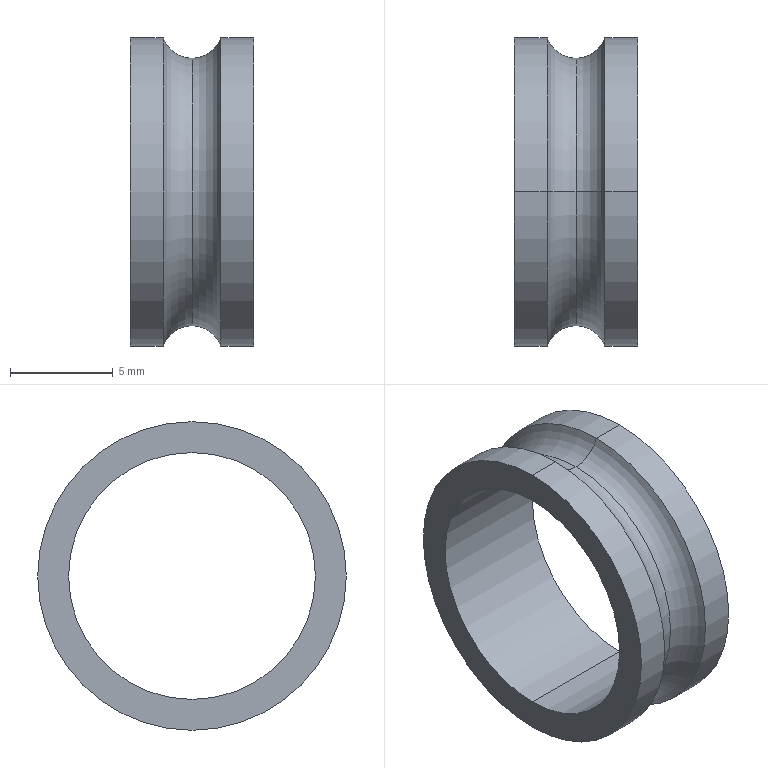Part | SolidWorks | features Revolution 1 | 1 solid | 12 faces | box 6 x 15 x 15 mm | volume 290.652 mm3 | cylinder 6 | torus 4 | plane 2 | commonest cylinder face diameters 15 x4 12 x2
STEP:
#1=CARTESIAN_POINT('',(1.6,0.,7.5));
#2=VERTEX_POINT('',#1);
#3=CARTESIAN_POINT('',(3.,0.,6.5));
#4=VERTEX_POINT('',#3);
#5=CARTESIAN_POINT('',(3.,0.,7.98));
#6=DIRECTION('',(0.,-1.,0.));
#7=DIRECTION('',(0.,0.,-1.));
#8=AXIS2_PLACEMENT_3D('',#5,#6,#7);
#9=CIRCLE('',#8,1.48);
#10=EDGE_CURVE('',#2,#4,#9,.T.);
#11=ORIENTED_EDGE('',*,*,#10,.T.);
#12=CARTESIAN_POINT('',(3.,0.,-6.5));
#13=VERTEX_POINT('',#12);
#14=CARTESIAN_POINT('',(3.,0.,0.));
#15=DIRECTION('',(-1.,0.,0.));
#16=DIRECTION('',(0.,0.,1.));
#17=AXIS2_PLACEMENT_3D('',#14,#15,#16);
#18=CIRCLE('',#17,6.5);
#19=EDGE_CURVE('',#4,#13,#18,.T.);
#20=ORIENTED_EDGE('',*,*,#19,.T.);
#21=CARTESIAN_POINT('',(1.6,0.,-7.5));
#22=VERTEX_POINT('',#21);
#23=CARTESIAN_POINT('',(3.,0.,-7.98));
#24=DIRECTION('',(0.,1.,0.));
#25=DIRECTION('',(0.,0.,1.));
#26=AXIS2_PLACEMENT_3D('',#23,#24,#25);
#27=CIRCLE('',#26,1.48);
#28=EDGE_CURVE('',#22,#13,#27,.T.);
#29=ORIENTED_EDGE('',*,*,#28,.F.);
#30=CARTESIAN_POINT('',(1.6,0.,0.));
#31=DIRECTION('',(-1.,0.,0.));
#32=DIRECTION('',(0.,0.,1.));
#33=AXIS2_PLACEMENT_3D('',#30,#31,#32);
#34=CIRCLE('',#33,7.5);
#35=EDGE_CURVE('',#2,#22,#34,.T.);
#36=ORIENTED_EDGE('',*,*,#35,.F.);
#37=EDGE_LOOP('',(#11,#20,#29,#36));
#38=FACE_OUTER_BOUND('',#37,.T.);
#39=CARTESIAN_POINT('',(3.,0.,0.));
#40=DIRECTION('',(-1.,0.,0.));
#41=DIRECTION('',(0.,0.,1.));
#42=AXIS2_PLACEMENT_3D('',#39,#40,#41);
#43=TOROIDAL_SURFACE('',#42,7.98,1.48);
#44=ADVANCED_FACE('',(#38),#43,.F.);
#45=ORIENTED_EDGE('',*,*,#28,.T.);
#46=CARTESIAN_POINT('',(3.,0.,0.));
#47=DIRECTION('',(-1.,0.,0.));
#48=DIRECTION('',(0.,0.,1.));
#49=AXIS2_PLACEMENT_3D('',#46,#47,#48);
#50=CIRCLE('',#49,6.5);
#51=EDGE_CURVE('',#13,#4,#50,.T.);
#52=ORIENTED_EDGE('',*,*,#51,.T.);
#53=ORIENTED_EDGE('',*,*,#10,.F.);
#54=CARTESIAN_POINT('',(1.6,0.,0.));
#55=DIRECTION('',(-1.,0.,0.));
#56=DIRECTION('',(0.,0.,1.));
#57=AXIS2_PLACEMENT_3D('',#54,#55,#56);
#58=CIRCLE('',#57,7.5);
#59=EDGE_CURVE('',#22,#2,#58,.T.);
#60=ORIENTED_EDGE('',*,*,#59,.F.);
#61=EDGE_LOOP('',(#45,#52,#53,#60));
#62=FACE_OUTER_BOUND('',#61,.T.);
#63=CARTESIAN_POINT('',(3.,0.,0.));
#64=DIRECTION('',(-1.,0.,0.));
#65=DIRECTION('',(0.,0.,1.));
#66=AXIS2_PLACEMENT_3D('',#63,#64,#65);
#67=TOROIDAL_SURFACE('',#66,7.98,1.48);
#68=ADVANCED_FACE('',(#62),#67,.F.);
#69=ORIENTED_EDGE('',*,*,#35,.T.);
#70=CARTESIAN_POINT('',(0.,0.,-7.5));
#71=VERTEX_POINT('',#70);
#72=CARTESIAN_POINT('',(0.,0.,-7.5));
#73=DIRECTION('',(-1.,0.,0.));
#74=VECTOR('',#73,1000.);
#75=LINE('',#72,#74);
#76=EDGE_CURVE('',#22,#71,#75,.T.);
#77=ORIENTED_EDGE('',*,*,#76,.T.);
#78=CARTESIAN_POINT('',(0.,0.,7.5));
#79=VERTEX_POINT('',#78);
#80=CARTESIAN_POINT('',(0.,0.,0.));
#81=DIRECTION('',(-1.,0.,0.));
#82=DIRECTION('',(0.,0.,1.));
#83=AXIS2_PLACEMENT_3D('',#80,#81,#82);
#84=CIRCLE('',#83,7.5);
#85=EDGE_CURVE('',#79,#71,#84,.T.);
#86=ORIENTED_EDGE('',*,*,#85,.F.);
#87=CARTESIAN_POINT('',(0.,0.,7.5));
#88=DIRECTION('',(-1.,0.,0.));
#89=VECTOR('',#88,1000.);
#90=LINE('',#87,#89);
#91=EDGE_CURVE('',#2,#79,#90,.T.);
#92=ORIENTED_EDGE('',*,*,#91,.F.);
#93=EDGE_LOOP('',(#69,#77,#86,#92));
#94=FACE_OUTER_BOUND('',#93,.T.);
#95=CARTESIAN_POINT('',(0.,0.,0.));
#96=DIRECTION('',(-1.,0.,0.));
#97=DIRECTION('',(0.,0.,1.));
#98=AXIS2_PLACEMENT_3D('',#95,#96,#97);
#99=CYLINDRICAL_SURFACE('',#98,7.5);
#100=ADVANCED_FACE('',(#94),#99,.T.);
#101=ORIENTED_EDGE('',*,*,#51,.F.);
#102=CARTESIAN_POINT('',(4.4,0.,-7.5));
#103=VERTEX_POINT('',#102);
#104=CARTESIAN_POINT('',(3.,0.,-7.98));
#105=DIRECTION('',(0.,1.,0.));
#106=DIRECTION('',(0.,0.,1.));
#107=AXIS2_PLACEMENT_3D('',#104,#105,#106);
#108=CIRCLE('',#107,1.48);
#109=EDGE_CURVE('',#13,#103,#108,.T.);
#110=ORIENTED_EDGE('',*,*,#109,.T.);
#111=CARTESIAN_POINT('',(4.4,0.,7.5));
#112=VERTEX_POINT('',#111);
#113=CARTESIAN_POINT('',(4.4,0.,0.));
#114=DIRECTION('',(-1.,0.,0.));
#115=DIRECTION('',(0.,0.,1.));
#116=AXIS2_PLACEMENT_3D('',#113,#114,#115);
#117=CIRCLE('',#116,7.5);
#118=EDGE_CURVE('',#103,#112,#117,.T.);
#119=ORIENTED_EDGE('',*,*,#118,.T.);
#120=CARTESIAN_POINT('',(3.,0.,7.98));
#121=DIRECTION('',(0.,-1.,0.));
#122=DIRECTION('',(0.,0.,-1.));
#123=AXIS2_PLACEMENT_3D('',#120,#121,#122);
#124=CIRCLE('',#123,1.48);
#125=EDGE_CURVE('',#4,#112,#124,.T.);
#126=ORIENTED_EDGE('',*,*,#125,.F.);
#127=EDGE_LOOP('',(#101,#110,#119,#126));
#128=FACE_OUTER_BOUND('',#127,.T.);
#129=CARTESIAN_POINT('',(3.,0.,0.));
#130=DIRECTION('',(-1.,0.,0.));
#131=DIRECTION('',(0.,0.,1.));
#132=AXIS2_PLACEMENT_3D('',#129,#130,#131);
#133=TOROIDAL_SURFACE('',#132,7.98,1.48);
#134=ADVANCED_FACE('',(#128),#133,.F.);
#135=CARTESIAN_POINT('',(6.,0.,7.5));
#136=VERTEX_POINT('',#135);
#137=CARTESIAN_POINT('',(6.,0.,-7.5));
#138=VERTEX_POINT('',#137);
#139=CARTESIAN_POINT('',(6.,0.,0.));
#140=DIRECTION('',(-1.,0.,0.));
#141=DIRECTION('',(0.,0.,1.));
#142=AXIS2_PLACEMENT_3D('',#139,#140,#141);
#143=CIRCLE('',#142,7.5);
#144=EDGE_CURVE('',#136,#138,#143,.T.);
#145=ORIENTED_EDGE('',*,*,#144,.T.);
#146=CARTESIAN_POINT('',(0.,0.,-7.5));
#147=DIRECTION('',(-1.,0.,0.));
#148=VECTOR('',#147,1000.);
#149=LINE('',#146,#148);
#150=EDGE_CURVE('',#138,#103,#149,.T.);
#151=ORIENTED_EDGE('',*,*,#150,.T.);
#152=CARTESIAN_POINT('',(4.4,0.,0.));
#153=DIRECTION('',(-1.,0.,0.));
#154=DIRECTION('',(0.,0.,1.));
#155=AXIS2_PLACEMENT_3D('',#152,#153,#154);
#156=CIRCLE('',#155,7.5);
#157=EDGE_CURVE('',#112,#103,#156,.T.);
#158=ORIENTED_EDGE('',*,*,#157,.F.);
#159=CARTESIAN_POINT('',(0.,0.,7.5));
#160=DIRECTION('',(-1.,0.,0.));
#161=VECTOR('',#160,1000.);
#162=LINE('',#159,#161);
#163=EDGE_CURVE('',#136,#112,#162,.T.);
#164=ORIENTED_EDGE('',*,*,#163,.F.);
#165=EDGE_LOOP('',(#145,#151,#158,#164));
#166=FACE_OUTER_BOUND('',#165,.T.);
#167=CARTESIAN_POINT('',(0.,0.,0.));
#168=DIRECTION('',(-1.,0.,0.));
#169=DIRECTION('',(0.,0.,1.));
#170=AXIS2_PLACEMENT_3D('',#167,#168,#169);
#171=CYLINDRICAL_SURFACE('',#170,7.5);
#172=ADVANCED_FACE('',(#166),#171,.T.);
#173=CARTESIAN_POINT('',(6.,0.,-6.));
#174=VERTEX_POINT('',#173);
#175=CARTESIAN_POINT('',(6.,0.,6.));
#176=VERTEX_POINT('',#175);
#177=CARTESIAN_POINT('',(6.,0.,0.));
#178=DIRECTION('',(-1.,0.,0.));
#179=DIRECTION('',(0.,0.,1.));
#180=AXIS2_PLACEMENT_3D('',#177,#178,#179);
#181=CIRCLE('',#180,6.);
#182=EDGE_CURVE('',#174,#176,#181,.T.);
#183=ORIENTED_EDGE('',*,*,#182,.F.);
#184=CARTESIAN_POINT('',(0.,0.,-6.));
#185=VERTEX_POINT('',#184);
#186=CARTESIAN_POINT('',(0.,0.,-6.));
#187=DIRECTION('',(-1.,0.,0.));
#188=VECTOR('',#187,1000.);
#189=LINE('',#186,#188);
#190=EDGE_CURVE('',#174,#185,#189,.T.);
#191=ORIENTED_EDGE('',*,*,#190,.T.);
#192=CARTESIAN_POINT('',(0.,0.,6.));
#193=VERTEX_POINT('',#192);
#194=CARTESIAN_POINT('',(0.,0.,0.));
#195=DIRECTION('',(-1.,0.,0.));
#196=DIRECTION('',(0.,0.,1.));
#197=AXIS2_PLACEMENT_3D('',#194,#195,#196);
#198=CIRCLE('',#197,6.);
#199=EDGE_CURVE('',#185,#193,#198,.T.);
#200=ORIENTED_EDGE('',*,*,#199,.T.);
#201=CARTESIAN_POINT('',(0.,0.,6.));
#202=DIRECTION('',(-1.,0.,0.));
#203=VECTOR('',#202,1000.);
#204=LINE('',#201,#203);
#205=EDGE_CURVE('',#176,#193,#204,.T.);
#206=ORIENTED_EDGE('',*,*,#205,.F.);
#207=EDGE_LOOP('',(#183,#191,#200,#206));
#208=FACE_OUTER_BOUND('',#207,.T.);
#209=CARTESIAN_POINT('',(0.,0.,0.));
#210=DIRECTION('',(-1.,0.,0.));
#211=DIRECTION('',(0.,0.,1.));
#212=AXIS2_PLACEMENT_3D('',#209,#210,#211);
#213=CYLINDRICAL_SURFACE('',#212,6.);
#214=ADVANCED_FACE('',(#208),#213,.F.);
#215=ORIENTED_EDGE('',*,*,#190,.F.);
#216=CARTESIAN_POINT('',(6.,0.,0.));
#217=DIRECTION('',(-1.,0.,0.));
#218=DIRECTION('',(0.,0.,1.));
#219=AXIS2_PLACEMENT_3D('',#216,#217,#218);
#220=CIRCLE('',#219,6.);
#221=EDGE_CURVE('',#176,#174,#220,.T.);
#222=ORIENTED_EDGE('',*,*,#221,.F.);
#223=ORIENTED_EDGE('',*,*,#205,.T.);
#224=CARTESIAN_POINT('',(0.,0.,0.));
#225=DIRECTION('',(-1.,0.,0.));
#226=DIRECTION('',(0.,0.,1.));
#227=AXIS2_PLACEMENT_3D('',#224,#225,#226);
#228=CIRCLE('',#227,6.);
#229=EDGE_CURVE('',#193,#185,#228,.T.);
#230=ORIENTED_EDGE('',*,*,#229,.T.);
#231=EDGE_LOOP('',(#215,#222,#223,#230));
#232=FACE_OUTER_BOUND('',#231,.T.);
#233=CARTESIAN_POINT('',(0.,0.,0.));
#234=DIRECTION('',(-1.,0.,0.));
#235=DIRECTION('',(0.,0.,1.));
#236=AXIS2_PLACEMENT_3D('',#233,#234,#235);
#237=CYLINDRICAL_SURFACE('',#236,6.);
#238=ADVANCED_FACE('',(#232),#237,.F.);
#239=ORIENTED_EDGE('',*,*,#144,.F.);
#240=CARTESIAN_POINT('',(6.,0.,0.));
#241=DIRECTION('',(-1.,0.,0.));
#242=DIRECTION('',(0.,0.,1.));
#243=AXIS2_PLACEMENT_3D('',#240,#241,#242);
#244=CIRCLE('',#243,7.5);
#245=EDGE_CURVE('',#138,#136,#244,.T.);
#246=ORIENTED_EDGE('',*,*,#245,.F.);
#247=EDGE_LOOP('',(#239,#246));
#248=FACE_OUTER_BOUND('',#247,.T.);
#249=ORIENTED_EDGE('',*,*,#221,.T.);
#250=ORIENTED_EDGE('',*,*,#182,.T.);
#251=EDGE_LOOP('',(#249,#250));
#252=FACE_BOUND('',#251,.T.);
#253=CARTESIAN_POINT('',(6.,7.5,0.));
#254=DIRECTION('',(-1.,0.,0.));
#255=DIRECTION('',(0.,0.,1.));
#256=AXIS2_PLACEMENT_3D('',#253,#254,#255);
#257=PLANE('',#256);
#258=ADVANCED_FACE('',(#248,#252),#257,.F.);
#259=ORIENTED_EDGE('',*,*,#150,.F.);
#260=ORIENTED_EDGE('',*,*,#245,.T.);
#261=ORIENTED_EDGE('',*,*,#163,.T.);
#262=ORIENTED_EDGE('',*,*,#118,.F.);
#263=EDGE_LOOP('',(#259,#260,#261,#262));
#264=FACE_OUTER_BOUND('',#263,.T.);
#265=CARTESIAN_POINT('',(0.,0.,0.));
#266=DIRECTION('',(-1.,0.,0.));
#267=DIRECTION('',(0.,0.,1.));
#268=AXIS2_PLACEMENT_3D('',#265,#266,#267);
#269=CYLINDRICAL_SURFACE('',#268,7.5);
#270=ADVANCED_FACE('',(#264),#269,.T.);
#271=ORIENTED_EDGE('',*,*,#19,.F.);
#272=ORIENTED_EDGE('',*,*,#125,.T.);
#273=ORIENTED_EDGE('',*,*,#157,.T.);
#274=ORIENTED_EDGE('',*,*,#109,.F.);
#275=EDGE_LOOP('',(#271,#272,#273,#274));
#276=FACE_OUTER_BOUND('',#275,.T.);
#277=CARTESIAN_POINT('',(3.,0.,0.));
#278=DIRECTION('',(-1.,0.,0.));
#279=DIRECTION('',(0.,0.,1.));
#280=AXIS2_PLACEMENT_3D('',#277,#278,#279);
#281=TOROIDAL_SURFACE('',#280,7.98,1.48);
#282=ADVANCED_FACE('',(#276),#281,.F.);
#283=ORIENTED_EDGE('',*,*,#76,.F.);
#284=ORIENTED_EDGE('',*,*,#59,.T.);
#285=ORIENTED_EDGE('',*,*,#91,.T.);
#286=CARTESIAN_POINT('',(0.,0.,0.));
#287=DIRECTION('',(-1.,0.,0.));
#288=DIRECTION('',(0.,0.,1.));
#289=AXIS2_PLACEMENT_3D('',#286,#287,#288);
#290=CIRCLE('',#289,7.5);
#291=EDGE_CURVE('',#71,#79,#290,.T.);
#292=ORIENTED_EDGE('',*,*,#291,.F.);
#293=EDGE_LOOP('',(#283,#284,#285,#292));
#294=FACE_OUTER_BOUND('',#293,.T.);
#295=CARTESIAN_POINT('',(0.,0.,0.));
#296=DIRECTION('',(-1.,0.,0.));
#297=DIRECTION('',(0.,0.,1.));
#298=AXIS2_PLACEMENT_3D('',#295,#296,#297);
#299=CYLINDRICAL_SURFACE('',#298,7.5);
#300=ADVANCED_FACE('',(#294),#299,.T.);
#301=ORIENTED_EDGE('',*,*,#229,.F.);
#302=ORIENTED_EDGE('',*,*,#199,.F.);
#303=EDGE_LOOP('',(#301,#302));
#304=FACE_BOUND('',#303,.T.);
#305=ORIENTED_EDGE('',*,*,#85,.T.);
#306=ORIENTED_EDGE('',*,*,#291,.T.);
#307=EDGE_LOOP('',(#305,#306));
#308=FACE_OUTER_BOUND('',#307,.T.);
#309=CARTESIAN_POINT('',(0.,6.,0.));
#310=DIRECTION('',(1.,0.,0.));
#311=DIRECTION('',(0.,0.,-1.));
#312=AXIS2_PLACEMENT_3D('',#309,#310,#311);
#313=PLANE('',#312);
#314=ADVANCED_FACE('',(#304,#308),#313,.F.);
#315=CLOSED_SHELL('',(#44,#68,#100,#134,#172,#214,#238,#258,#270,#282,#300,#314));
#316=MANIFOLD_SOLID_BREP('',#315);
#317=CARTESIAN_POINT('',(0.,0.,0.));
#318=DIRECTION('',(0.,0.,1.));
#319=DIRECTION('',(1.,0.,0.));
#320=AXIS2_PLACEMENT_3D('',#317,#318,#319);
#321=(LENGTH_UNIT()NAMED_UNIT(*)SI_UNIT(.MILLI.,.METRE.));
#322=UNCERTAINTY_MEASURE_WITH_UNIT(LENGTH_MEASURE(0.00001),#321,'','');
#323=(NAMED_UNIT(*)PLANE_ANGLE_UNIT()SI_UNIT($,.RADIAN.));
#324=(NAMED_UNIT(*)SI_UNIT($,.STERADIAN.)SOLID_ANGLE_UNIT());
#325=(GEOMETRIC_REPRESENTATION_CONTEXT(3)GLOBAL_UNCERTAINTY_ASSIGNED_CONTEXT((#322))GLOBAL_UNIT_ASSIGNED_CONTEXT((#321,#323,#324))REPRESENTATION_CONTEXT('',''));
#326=ADVANCED_BREP_SHAPE_REPRESENTATION('',(#316,#320),#325);